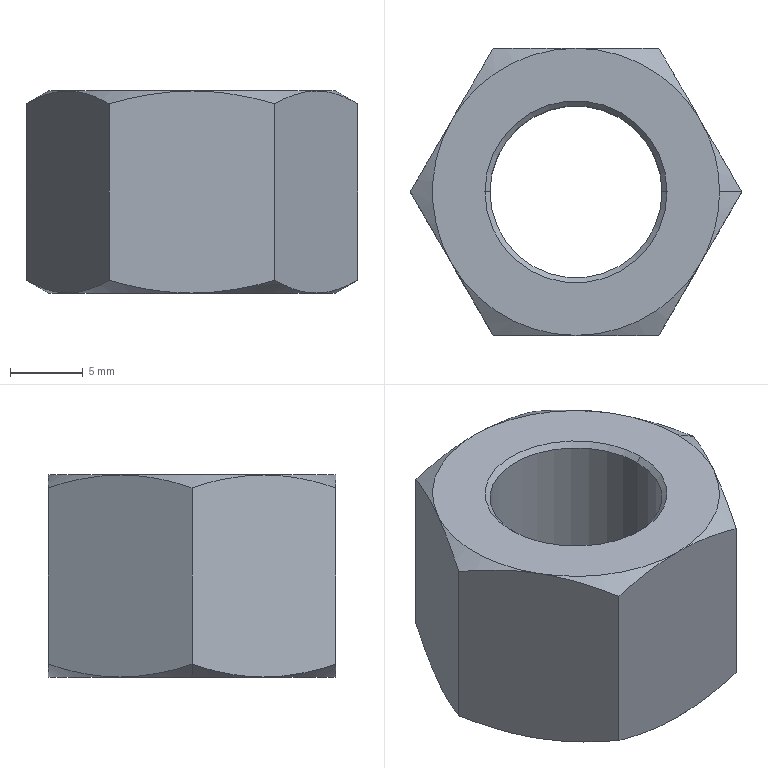Part | SolidWorks | features Cut 2, Chamfer 1, Extrusion 1 | 1 solid | 28 faces | box 22.8 x 19.745 x 13.9 mm | volume 3143 mm3 | cone 18 | plane 8 | cylinder 2 | commonest cylinder face diameters 11.835 x2
STEP:
#1=CARTESIAN_POINT('',(-5.917,0.,13.553));
#2=VERTEX_POINT('',#1);
#3=CARTESIAN_POINT('',(5.917,0.,13.553));
#4=VERTEX_POINT('',#3);
#5=CARTESIAN_POINT('',(0.,0.,13.553));
#6=DIRECTION('',(0.,0.,1.));
#7=DIRECTION('',(1.,0.,0.));
#8=AXIS2_PLACEMENT_3D('',#5,#6,#7);
#9=CIRCLE('',#8,5.917);
#10=EDGE_CURVE('',#2,#4,#9,.T.);
#11=ORIENTED_EDGE('',*,*,#10,.F.);
#12=CARTESIAN_POINT('',(-6.265,0.,13.9));
#13=VERTEX_POINT('',#12);
#14=CARTESIAN_POINT('',(-5.917,0.,13.553));
#15=DIRECTION('',(-0.7071,0.,0.7071));
#16=VECTOR('',#15,1000.);
#17=LINE('',#14,#16);
#18=EDGE_CURVE('',#2,#13,#17,.T.);
#19=ORIENTED_EDGE('',*,*,#18,.T.);
#20=CARTESIAN_POINT('',(6.265,0.,13.9));
#21=VERTEX_POINT('',#20);
#22=CARTESIAN_POINT('',(0.,0.,13.9));
#23=DIRECTION('',(0.,0.,-1.));
#24=DIRECTION('',(1.,0.,0.));
#25=AXIS2_PLACEMENT_3D('',#22,#23,#24);
#26=CIRCLE('',#25,6.265);
#27=EDGE_CURVE('',#21,#13,#26,.T.);
#28=ORIENTED_EDGE('',*,*,#27,.F.);
#29=CARTESIAN_POINT('',(5.917,0.,13.553));
#30=DIRECTION('',(0.7071,0.,0.7071));
#31=VECTOR('',#30,1000.);
#32=LINE('',#29,#31);
#33=EDGE_CURVE('',#4,#21,#32,.T.);
#34=ORIENTED_EDGE('',*,*,#33,.F.);
#35=EDGE_LOOP('',(#11,#19,#28,#34));
#36=FACE_OUTER_BOUND('',#35,.T.);
#37=CARTESIAN_POINT('',(0.,0.,13.553));
#38=DIRECTION('',(0.,0.,1.));
#39=DIRECTION('',(1.,0.,0.));
#40=AXIS2_PLACEMENT_3D('',#37,#38,#39);
#41=CONICAL_SURFACE('',#40,5.917,0.7854);
#42=ADVANCED_FACE('',(#36),#41,.F.);
#43=CARTESIAN_POINT('',(5.917,0.,0.3475));
#44=VERTEX_POINT('',#43);
#45=CARTESIAN_POINT('',(-5.917,0.,0.3475));
#46=VERTEX_POINT('',#45);
#47=CARTESIAN_POINT('',(0.,0.,0.3475));
#48=DIRECTION('',(0.,0.,-1.));
#49=DIRECTION('',(1.,0.,0.));
#50=AXIS2_PLACEMENT_3D('',#47,#48,#49);
#51=CIRCLE('',#50,5.917);
#52=EDGE_CURVE('',#44,#46,#51,.T.);
#53=ORIENTED_EDGE('',*,*,#52,.F.);
#54=CARTESIAN_POINT('',(6.265,0.,0.));
#55=VERTEX_POINT('',#54);
#56=CARTESIAN_POINT('',(6.265,0.,0.));
#57=DIRECTION('',(0.7071,0.,-0.7071));
#58=VECTOR('',#57,1000.);
#59=LINE('',#56,#58);
#60=EDGE_CURVE('',#44,#55,#59,.T.);
#61=ORIENTED_EDGE('',*,*,#60,.T.);
#62=CARTESIAN_POINT('',(-6.265,0.,0.));
#63=VERTEX_POINT('',#62);
#64=CARTESIAN_POINT('',(0.,0.,0.));
#65=DIRECTION('',(0.,0.,1.));
#66=DIRECTION('',(1.,0.,0.));
#67=AXIS2_PLACEMENT_3D('',#64,#65,#66);
#68=CIRCLE('',#67,6.265);
#69=EDGE_CURVE('',#63,#55,#68,.T.);
#70=ORIENTED_EDGE('',*,*,#69,.F.);
#71=CARTESIAN_POINT('',(-6.265,0.,0.));
#72=DIRECTION('',(-0.7071,0.,-0.7071));
#73=VECTOR('',#72,1000.);
#74=LINE('',#71,#73);
#75=EDGE_CURVE('',#46,#63,#74,.T.);
#76=ORIENTED_EDGE('',*,*,#75,.F.);
#77=EDGE_LOOP('',(#53,#61,#70,#76));
#78=FACE_OUTER_BOUND('',#77,.T.);
#79=CARTESIAN_POINT('',(0.,0.,0.));
#80=DIRECTION('',(0.,0.,-1.));
#81=DIRECTION('',(-1.,0.,0.));
#82=AXIS2_PLACEMENT_3D('',#79,#80,#81);
#83=CONICAL_SURFACE('',#82,6.265,0.7854);
#84=ADVANCED_FACE('',(#78),#83,.F.);
#85=CARTESIAN_POINT('',(9.873,0.,13.9));
#86=VERTEX_POINT('',#85);
#87=CARTESIAN_POINT('',(8.55,4.936,13.9));
#88=VERTEX_POINT('',#87);
#89=CARTESIAN_POINT('',(0.,0.,13.9));
#90=DIRECTION('',(0.,0.,1.));
#91=DIRECTION('',(1.,0.,0.));
#92=AXIS2_PLACEMENT_3D('',#89,#90,#91);
#93=CIRCLE('',#92,9.873);
#94=EDGE_CURVE('',#86,#88,#93,.T.);
#95=ORIENTED_EDGE('',*,*,#94,.F.);
#96=CARTESIAN_POINT('',(11.4,0.,13.018));
#97=VERTEX_POINT('',#96);
#98=CARTESIAN_POINT('',(9.873,0.,13.9));
#99=DIRECTION('',(0.866,0.,-0.5));
#100=VECTOR('',#99,1000.);
#101=LINE('',#98,#100);
#102=EDGE_CURVE('',#86,#97,#101,.T.);
#103=ORIENTED_EDGE('',*,*,#102,.T.);
#104=CARTESIAN_POINT('',(11.4,0.,13.018));
#105=CARTESIAN_POINT('',(10.934,0.8075,13.287));
#106=CARTESIAN_POINT('',(10.464,1.621,13.509));
#107=CARTESIAN_POINT('',(9.515,3.265,13.816));
#108=CARTESIAN_POINT('',(9.036,4.095,13.9));
#109=CARTESIAN_POINT('',(8.55,4.936,13.9));
#110=B_SPLINE_CURVE_WITH_KNOTS('',3,(#104,#105,#106,#107,#108,#109),.UNSPECIFIED.,.F.,.F.,(4,2,4),(0.000000238,0.002884,0.005768),.UNSPECIFIED.);
#111=EDGE_CURVE('',#97,#88,#110,.T.);
#112=ORIENTED_EDGE('',*,*,#111,.T.);
#113=EDGE_LOOP('',(#95,#103,#112));
#114=FACE_OUTER_BOUND('',#113,.T.);
#115=CARTESIAN_POINT('',(0.,0.,13.9));
#116=DIRECTION('',(0.,0.,-1.));
#117=DIRECTION('',(1.,0.,0.));
#118=AXIS2_PLACEMENT_3D('',#115,#116,#117);
#119=CONICAL_SURFACE('',#118,9.873,1.047);
#120=ADVANCED_FACE('',(#114),#119,.T.);
#121=CARTESIAN_POINT('',(-9.873,0.,0.));
#122=VERTEX_POINT('',#121);
#123=CARTESIAN_POINT('',(-8.55,4.936,0.));
#124=VERTEX_POINT('',#123);
#125=CARTESIAN_POINT('',(0.,0.,0.));
#126=DIRECTION('',(0.,0.,-1.));
#127=DIRECTION('',(-1.,0.,0.));
#128=AXIS2_PLACEMENT_3D('',#125,#126,#127);
#129=CIRCLE('',#128,9.873);
#130=EDGE_CURVE('',#122,#124,#129,.T.);
#131=ORIENTED_EDGE('',*,*,#130,.F.);
#132=CARTESIAN_POINT('',(-11.4,0.,0.8818));
#133=VERTEX_POINT('',#132);
#134=CARTESIAN_POINT('',(-9.873,0.,0.));
#135=DIRECTION('',(-0.866,0.,0.5));
#136=VECTOR('',#135,1000.);
#137=LINE('',#134,#136);
#138=EDGE_CURVE('',#122,#133,#137,.T.);
#139=ORIENTED_EDGE('',*,*,#138,.T.);
#140=CARTESIAN_POINT('',(-11.4,0.,0.8818));
#141=CARTESIAN_POINT('',(-10.934,0.8075,0.6126));
#142=CARTESIAN_POINT('',(-10.464,1.621,0.3909));
#143=CARTESIAN_POINT('',(-9.515,3.265,0.08404));
#144=CARTESIAN_POINT('',(-9.036,4.095,0.));
#145=CARTESIAN_POINT('',(-8.55,4.936,0.));
#146=B_SPLINE_CURVE_WITH_KNOTS('',3,(#140,#141,#142,#143,#144,#145),.UNSPECIFIED.,.F.,.F.,(4,2,4),(0.000000238,0.002884,0.005768),.UNSPECIFIED.);
#147=EDGE_CURVE('',#133,#124,#146,.T.);
#148=ORIENTED_EDGE('',*,*,#147,.T.);
#149=EDGE_LOOP('',(#131,#139,#148));
#150=FACE_OUTER_BOUND('',#149,.T.);
#151=CARTESIAN_POINT('',(0.,0.,0.));
#152=DIRECTION('',(0.,0.,1.));
#153=DIRECTION('',(-1.,0.,0.));
#154=AXIS2_PLACEMENT_3D('',#151,#152,#153);
#155=CONICAL_SURFACE('',#154,9.873,1.047);
#156=ADVANCED_FACE('',(#150),#155,.T.);
#157=ORIENTED_EDGE('',*,*,#10,.T.);
#158=CARTESIAN_POINT('',(5.917,0.,13.9));
#159=DIRECTION('',(0.,0.,-1.));
#160=VECTOR('',#159,1000.);
#161=LINE('',#158,#160);
#162=EDGE_CURVE('',#4,#44,#161,.T.);
#163=ORIENTED_EDGE('',*,*,#162,.T.);
#164=ORIENTED_EDGE('',*,*,#52,.T.);
#165=CARTESIAN_POINT('',(-5.917,0.,13.9));
#166=DIRECTION('',(0.,0.,-1.));
#167=VECTOR('',#166,1000.);
#168=LINE('',#165,#167);
#169=EDGE_CURVE('',#2,#46,#168,.T.);
#170=ORIENTED_EDGE('',*,*,#169,.F.);
#171=EDGE_LOOP('',(#157,#163,#164,#170));
#172=FACE_OUTER_BOUND('',#171,.T.);
#173=CARTESIAN_POINT('',(0.,0.,13.9));
#174=DIRECTION('',(0.,0.,-1.));
#175=DIRECTION('',(-1.,0.,0.));
#176=AXIS2_PLACEMENT_3D('',#173,#174,#175);
#177=CYLINDRICAL_SURFACE('',#176,5.917);
#178=ADVANCED_FACE('',(#172),#177,.F.);
#179=ORIENTED_EDGE('',*,*,#111,.F.);
#180=CARTESIAN_POINT('',(11.4,0.,0.8818));
#181=VERTEX_POINT('',#180);
#182=CARTESIAN_POINT('',(11.4,0.,13.9));
#183=DIRECTION('',(0.,0.,-1.));
#184=VECTOR('',#183,1000.);
#185=LINE('',#182,#184);
#186=EDGE_CURVE('',#97,#181,#185,.T.);
#187=ORIENTED_EDGE('',*,*,#186,.T.);
#188=CARTESIAN_POINT('',(8.55,4.936,0.));
#189=VERTEX_POINT('',#188);
#190=CARTESIAN_POINT('',(8.55,4.936,0.));
#191=CARTESIAN_POINT('',(8.792,4.517,0.));
#192=CARTESIAN_POINT('',(9.035,4.097,0.02084));
#193=CARTESIAN_POINT('',(9.515,3.264,0.1015));
#194=CARTESIAN_POINT('',(9.754,2.851,0.1612));
#195=CARTESIAN_POINT('',(10.466,1.618,0.3916));
#196=CARTESIAN_POINT('',(10.935,0.8055,0.6133));
#197=CARTESIAN_POINT('',(11.4,0.,0.8818));
#198=B_SPLINE_CURVE_WITH_KNOTS('',3,(#190,#191,#192,#193,#194,#195,#196,#197),.UNSPECIFIED.,.F.,.F.,(4,2,2,4),(0.005768,0.007204,0.008641,0.01151),.UNSPECIFIED.);
#199=EDGE_CURVE('',#189,#181,#198,.T.);
#200=ORIENTED_EDGE('',*,*,#199,.F.);
#201=CARTESIAN_POINT('',(5.7,9.873,0.8818));
#202=VERTEX_POINT('',#201);
#203=CARTESIAN_POINT('',(5.7,9.873,0.8818));
#204=CARTESIAN_POINT('',(6.166,9.065,0.6126));
#205=CARTESIAN_POINT('',(6.636,8.252,0.3909));
#206=CARTESIAN_POINT('',(7.585,6.608,0.08404));
#207=CARTESIAN_POINT('',(8.064,5.777,0.));
#208=CARTESIAN_POINT('',(8.55,4.936,0.));
#209=B_SPLINE_CURVE_WITH_KNOTS('',3,(#203,#204,#205,#206,#207,#208),.UNSPECIFIED.,.F.,.F.,(4,2,4),(0.000000238,0.002884,0.005768),.UNSPECIFIED.);
#210=EDGE_CURVE('',#202,#189,#209,.T.);
#211=ORIENTED_EDGE('',*,*,#210,.F.);
#212=CARTESIAN_POINT('',(5.7,9.873,13.018));
#213=VERTEX_POINT('',#212);
#214=CARTESIAN_POINT('',(5.7,9.873,13.9));
#215=DIRECTION('',(0.,0.,-1.));
#216=VECTOR('',#215,1000.);
#217=LINE('',#214,#216);
#218=EDGE_CURVE('',#213,#202,#217,.T.);
#219=ORIENTED_EDGE('',*,*,#218,.F.);
#220=CARTESIAN_POINT('',(8.55,4.936,13.9));
#221=CARTESIAN_POINT('',(8.308,5.355,13.9));
#222=CARTESIAN_POINT('',(8.065,5.776,13.879));
#223=CARTESIAN_POINT('',(7.585,6.609,13.799));
#224=CARTESIAN_POINT('',(7.346,7.022,13.739));
#225=CARTESIAN_POINT('',(6.634,8.255,13.508));
#226=CARTESIAN_POINT('',(6.165,9.067,13.287));
#227=CARTESIAN_POINT('',(5.7,9.873,13.018));
#228=B_SPLINE_CURVE_WITH_KNOTS('',3,(#220,#221,#222,#223,#224,#225,#226,#227),.UNSPECIFIED.,.F.,.F.,(4,2,2,4),(0.005768,0.007204,0.008641,0.01151),.UNSPECIFIED.);
#229=EDGE_CURVE('',#88,#213,#228,.T.);
#230=ORIENTED_EDGE('',*,*,#229,.F.);
#231=EDGE_LOOP('',(#179,#187,#200,#211,#219,#230));
#232=FACE_OUTER_BOUND('',#231,.T.);
#233=CARTESIAN_POINT('',(11.4,0.,13.9));
#234=DIRECTION('',(-0.866,-0.5,0.));
#235=DIRECTION('',(0.5,-0.866,0.));
#236=AXIS2_PLACEMENT_3D('',#233,#234,#235);
#237=PLANE('',#236);
#238=ADVANCED_FACE('',(#232),#237,.F.);
#239=CARTESIAN_POINT('',(0.,9.873,13.9));
#240=VERTEX_POINT('',#239);
#241=CARTESIAN_POINT('',(5.7,9.873,13.018));
#242=CARTESIAN_POINT('',(4.778,9.873,13.284));
#243=CARTESIAN_POINT('',(3.845,9.873,13.506));
#244=CARTESIAN_POINT('',(2.418,9.873,13.737));
#245=CARTESIAN_POINT('',(1.938,9.873,13.798));
#246=CARTESIAN_POINT('',(0.9674,9.873,13.879));
#247=CARTESIAN_POINT('',(0.4824,9.873,13.9));
#248=CARTESIAN_POINT('',(0.,9.873,13.9));
#249=B_SPLINE_CURVE_WITH_KNOTS('',3,(#241,#242,#243,#244,#245,#246,#247,#248),.UNSPECIFIED.,.F.,.F.,(4,2,2,4),(0.03412,0.03701,0.03845,0.03989),.UNSPECIFIED.);
#250=EDGE_CURVE('',#213,#240,#249,.T.);
#251=ORIENTED_EDGE('',*,*,#250,.F.);
#252=ORIENTED_EDGE('',*,*,#218,.T.);
#253=CARTESIAN_POINT('',(0.,9.873,0.));
#254=VERTEX_POINT('',#253);
#255=CARTESIAN_POINT('',(0.,9.873,0.));
#256=CARTESIAN_POINT('',(0.4824,9.873,0.));
#257=CARTESIAN_POINT('',(0.9674,9.873,0.02059));
#258=CARTESIAN_POINT('',(1.938,9.873,0.1021));
#259=CARTESIAN_POINT('',(2.418,9.873,0.1625));
#260=CARTESIAN_POINT('',(3.845,9.873,0.3942));
#261=CARTESIAN_POINT('',(4.778,9.873,0.6157));
#262=CARTESIAN_POINT('',(5.7,9.873,0.8818));
#263=B_SPLINE_CURVE_WITH_KNOTS('',3,(#255,#256,#257,#258,#259,#260,#261,#262),.UNSPECIFIED.,.F.,.F.,(4,2,2,4),(0.01627,0.01771,0.01915,0.02204),.UNSPECIFIED.);
#264=EDGE_CURVE('',#254,#202,#263,.T.);
#265=ORIENTED_EDGE('',*,*,#264,.F.);
#266=CARTESIAN_POINT('',(-5.7,9.873,0.8818));
#267=VERTEX_POINT('',#266);
#268=CARTESIAN_POINT('',(-5.7,9.873,0.8818));
#269=CARTESIAN_POINT('',(-4.772,9.873,0.6139));
#270=CARTESIAN_POINT('',(-3.823,9.873,0.3896));
#271=CARTESIAN_POINT('',(-1.921,9.873,0.08294));
#272=CARTESIAN_POINT('',(-0.9642,9.873,0.));
#273=CARTESIAN_POINT('',(0.,9.873,0.));
#274=B_SPLINE_CURVE_WITH_KNOTS('',3,(#268,#269,#270,#271,#272,#273),.UNSPECIFIED.,.F.,.F.,(4,2,4),(0.0105,0.01338,0.01627),.UNSPECIFIED.);
#275=EDGE_CURVE('',#267,#254,#274,.T.);
#276=ORIENTED_EDGE('',*,*,#275,.F.);
#277=CARTESIAN_POINT('',(-5.7,9.873,13.018));
#278=VERTEX_POINT('',#277);
#279=CARTESIAN_POINT('',(-5.7,9.873,13.9));
#280=DIRECTION('',(0.,0.,-1.));
#281=VECTOR('',#280,1000.);
#282=LINE('',#279,#281);
#283=EDGE_CURVE('',#278,#267,#282,.T.);
#284=ORIENTED_EDGE('',*,*,#283,.F.);
#285=CARTESIAN_POINT('',(0.,9.873,13.9));
#286=CARTESIAN_POINT('',(-0.9642,9.873,13.9));
#287=CARTESIAN_POINT('',(-1.921,9.873,13.817));
#288=CARTESIAN_POINT('',(-3.823,9.873,13.51));
#289=CARTESIAN_POINT('',(-4.772,9.873,13.286));
#290=CARTESIAN_POINT('',(-5.7,9.873,13.018));
#291=B_SPLINE_CURVE_WITH_KNOTS('',3,(#285,#286,#287,#288,#289,#290),.UNSPECIFIED.,.F.,.F.,(4,2,4),(0.03989,0.04277,0.04566),.UNSPECIFIED.);
#292=EDGE_CURVE('',#240,#278,#291,.T.);
#293=ORIENTED_EDGE('',*,*,#292,.F.);
#294=EDGE_LOOP('',(#251,#252,#265,#276,#284,#293));
#295=FACE_OUTER_BOUND('',#294,.T.);
#296=CARTESIAN_POINT('',(5.7,9.873,13.9));
#297=DIRECTION('',(0.,-1.,0.));
#298=DIRECTION('',(1.,0.,0.));
#299=AXIS2_PLACEMENT_3D('',#296,#297,#298);
#300=PLANE('',#299);
#301=ADVANCED_FACE('',(#295),#300,.F.);
#302=CARTESIAN_POINT('',(-8.55,4.936,13.9));
#303=VERTEX_POINT('',#302);
#304=CARTESIAN_POINT('',(-5.7,9.873,13.018));
#305=CARTESIAN_POINT('',(-6.166,9.065,13.287));
#306=CARTESIAN_POINT('',(-6.636,8.252,13.509));
#307=CARTESIAN_POINT('',(-7.585,6.608,13.816));
#308=CARTESIAN_POINT('',(-8.064,5.777,13.9));
#309=CARTESIAN_POINT('',(-8.55,4.936,13.9));
#310=B_SPLINE_CURVE_WITH_KNOTS('',3,(#304,#305,#306,#307,#308,#309),.UNSPECIFIED.,.F.,.F.,(4,2,4),(0.000000238,0.002884,0.005768),.UNSPECIFIED.);
#311=EDGE_CURVE('',#278,#303,#310,.T.);
#312=ORIENTED_EDGE('',*,*,#311,.F.);
#313=ORIENTED_EDGE('',*,*,#283,.T.);
#314=CARTESIAN_POINT('',(-8.55,4.936,0.));
#315=CARTESIAN_POINT('',(-8.308,5.355,0.));
#316=CARTESIAN_POINT('',(-8.065,5.776,0.02084));
#317=CARTESIAN_POINT('',(-7.585,6.609,0.1015));
#318=CARTESIAN_POINT('',(-7.346,7.022,0.1612));
#319=CARTESIAN_POINT('',(-6.634,8.255,0.3916));
#320=CARTESIAN_POINT('',(-6.165,9.067,0.6133));
#321=CARTESIAN_POINT('',(-5.7,9.873,0.8818));
#322=B_SPLINE_CURVE_WITH_KNOTS('',3,(#314,#315,#316,#317,#318,#319,#320,#321),.UNSPECIFIED.,.F.,.F.,(4,2,2,4),(0.005768,0.007204,0.008641,0.01151),.UNSPECIFIED.);
#323=EDGE_CURVE('',#124,#267,#322,.T.);
#324=ORIENTED_EDGE('',*,*,#323,.F.);
#325=ORIENTED_EDGE('',*,*,#147,.F.);
#326=CARTESIAN_POINT('',(-11.4,0.,13.018));
#327=VERTEX_POINT('',#326);
#328=CARTESIAN_POINT('',(-11.4,0.,13.9));
#329=DIRECTION('',(0.,0.,-1.));
#330=VECTOR('',#329,1000.);
#331=LINE('',#328,#330);
#332=EDGE_CURVE('',#327,#133,#331,.T.);
#333=ORIENTED_EDGE('',*,*,#332,.F.);
#334=CARTESIAN_POINT('',(-8.55,4.936,13.9));
#335=CARTESIAN_POINT('',(-8.792,4.517,13.9));
#336=CARTESIAN_POINT('',(-9.035,4.097,13.879));
#337=CARTESIAN_POINT('',(-9.515,3.264,13.799));
#338=CARTESIAN_POINT('',(-9.754,2.851,13.739));
#339=CARTESIAN_POINT('',(-10.466,1.618,13.508));
#340=CARTESIAN_POINT('',(-10.935,0.8055,13.287));
#341=CARTESIAN_POINT('',(-11.4,0.,13.018));
#342=B_SPLINE_CURVE_WITH_KNOTS('',3,(#334,#335,#336,#337,#338,#339,#340,#341),.UNSPECIFIED.,.F.,.F.,(4,2,2,4),(0.005768,0.007204,0.008641,0.01151),.UNSPECIFIED.);
#343=EDGE_CURVE('',#303,#327,#342,.T.);
#344=ORIENTED_EDGE('',*,*,#343,.F.);
#345=EDGE_LOOP('',(#312,#313,#324,#325,#333,#344));
#346=FACE_OUTER_BOUND('',#345,.T.);
#347=CARTESIAN_POINT('',(-5.7,9.873,13.9));
#348=DIRECTION('',(0.866,-0.5,0.));
#349=DIRECTION('',(0.5,0.866,0.));
#350=AXIS2_PLACEMENT_3D('',#347,#348,#349);
#351=PLANE('',#350);
#352=ADVANCED_FACE('',(#346),#351,.F.);
#353=CARTESIAN_POINT('',(-8.55,-4.936,13.9));
#354=VERTEX_POINT('',#353);
#355=CARTESIAN_POINT('',(-11.4,0.,13.018));
#356=CARTESIAN_POINT('',(-10.934,-0.8075,13.287));
#357=CARTESIAN_POINT('',(-10.464,-1.621,13.509));
#358=CARTESIAN_POINT('',(-9.515,-3.265,13.816));
#359=CARTESIAN_POINT('',(-9.036,-4.095,13.9));
#360=CARTESIAN_POINT('',(-8.55,-4.936,13.9));
#361=B_SPLINE_CURVE_WITH_KNOTS('',3,(#355,#356,#357,#358,#359,#360),.UNSPECIFIED.,.F.,.F.,(4,2,4),(0.000000238,0.002884,0.005768),.UNSPECIFIED.);
#362=EDGE_CURVE('',#327,#354,#361,.T.);
#363=ORIENTED_EDGE('',*,*,#362,.F.);
#364=ORIENTED_EDGE('',*,*,#332,.T.);
#365=CARTESIAN_POINT('',(-8.55,-4.936,0.));
#366=VERTEX_POINT('',#365);
#367=CARTESIAN_POINT('',(-8.55,-4.936,0.));
#368=CARTESIAN_POINT('',(-8.792,-4.517,0.));
#369=CARTESIAN_POINT('',(-9.035,-4.097,0.02084));
#370=CARTESIAN_POINT('',(-9.515,-3.264,0.1015));
#371=CARTESIAN_POINT('',(-9.754,-2.851,0.1612));
#372=CARTESIAN_POINT('',(-10.466,-1.618,0.3916));
#373=CARTESIAN_POINT('',(-10.935,-0.8055,0.6133));
#374=CARTESIAN_POINT('',(-11.4,0.,0.8818));
#375=B_SPLINE_CURVE_WITH_KNOTS('',3,(#367,#368,#369,#370,#371,#372,#373,#374),.UNSPECIFIED.,.F.,.F.,(4,2,2,4),(0.005768,0.007204,0.008641,0.01151),.UNSPECIFIED.);
#376=EDGE_CURVE('',#366,#133,#375,.T.);
#377=ORIENTED_EDGE('',*,*,#376,.F.);
#378=CARTESIAN_POINT('',(-5.7,-9.873,0.8818));
#379=VERTEX_POINT('',#378);
#380=CARTESIAN_POINT('',(-5.7,-9.873,0.8818));
#381=CARTESIAN_POINT('',(-6.166,-9.065,0.6126));
#382=CARTESIAN_POINT('',(-6.636,-8.252,0.3909));
#383=CARTESIAN_POINT('',(-7.585,-6.608,0.08404));
#384=CARTESIAN_POINT('',(-8.064,-5.777,0.));
#385=CARTESIAN_POINT('',(-8.55,-4.936,0.));
#386=B_SPLINE_CURVE_WITH_KNOTS('',3,(#380,#381,#382,#383,#384,#385),.UNSPECIFIED.,.F.,.F.,(4,2,4),(0.000000238,0.002884,0.005768),.UNSPECIFIED.);
#387=EDGE_CURVE('',#379,#366,#386,.T.);
#388=ORIENTED_EDGE('',*,*,#387,.F.);
#389=CARTESIAN_POINT('',(-5.7,-9.873,13.018));
#390=VERTEX_POINT('',#389);
#391=CARTESIAN_POINT('',(-5.7,-9.873,13.9));
#392=DIRECTION('',(0.,0.,-1.));
#393=VECTOR('',#392,1000.);
#394=LINE('',#391,#393);
#395=EDGE_CURVE('',#390,#379,#394,.T.);
#396=ORIENTED_EDGE('',*,*,#395,.F.);
#397=CARTESIAN_POINT('',(-8.55,-4.936,13.9));
#398=CARTESIAN_POINT('',(-8.308,-5.355,13.9));
#399=CARTESIAN_POINT('',(-8.065,-5.776,13.879));
#400=CARTESIAN_POINT('',(-7.585,-6.609,13.799));
#401=CARTESIAN_POINT('',(-7.346,-7.022,13.739));
#402=CARTESIAN_POINT('',(-6.634,-8.255,13.508));
#403=CARTESIAN_POINT('',(-6.165,-9.067,13.287));
#404=CARTESIAN_POINT('',(-5.7,-9.873,13.018));
#405=B_SPLINE_CURVE_WITH_KNOTS('',3,(#397,#398,#399,#400,#401,#402,#403,#404),.UNSPECIFIED.,.F.,.F.,(4,2,2,4),(0.005768,0.007204,0.008641,0.01151),.UNSPECIFIED.);
#406=EDGE_CURVE('',#354,#390,#405,.T.);
#407=ORIENTED_EDGE('',*,*,#406,.F.);
#408=EDGE_LOOP('',(#363,#364,#377,#388,#396,#407));
#409=FACE_OUTER_BOUND('',#408,.T.);
#410=CARTESIAN_POINT('',(-11.4,0.,13.9));
#411=DIRECTION('',(0.866,0.5,0.));
#412=DIRECTION('',(-0.5,0.866,0.));
#413=AXIS2_PLACEMENT_3D('',#410,#411,#412);
#414=PLANE('',#413);
#415=ADVANCED_FACE('',(#409),#414,.F.);
#416=CARTESIAN_POINT('',(0.,-9.873,13.9));
#417=VERTEX_POINT('',#416);
#418=CARTESIAN_POINT('',(-5.7,-9.873,13.018));
#419=CARTESIAN_POINT('',(-4.772,-9.873,13.286));
#420=CARTESIAN_POINT('',(-3.823,-9.873,13.51));
#421=CARTESIAN_POINT('',(-1.921,-9.873,13.817));
#422=CARTESIAN_POINT('',(-0.9642,-9.873,13.9));
#423=CARTESIAN_POINT('',(0.,-9.873,13.9));
#424=B_SPLINE_CURVE_WITH_KNOTS('',3,(#418,#419,#420,#421,#422,#423),.UNSPECIFIED.,.F.,.F.,(4,2,4),(0.0105,0.01338,0.01627),.UNSPECIFIED.);
#425=EDGE_CURVE('',#390,#417,#424,.T.);
#426=ORIENTED_EDGE('',*,*,#425,.F.);
#427=ORIENTED_EDGE('',*,*,#395,.T.);
#428=CARTESIAN_POINT('',(0.,-9.873,0.));
#429=VERTEX_POINT('',#428);
#430=CARTESIAN_POINT('',(0.,-9.873,0.));
#431=CARTESIAN_POINT('',(-0.9642,-9.873,0.));
#432=CARTESIAN_POINT('',(-1.921,-9.873,0.08294));
#433=CARTESIAN_POINT('',(-3.823,-9.873,0.3896));
#434=CARTESIAN_POINT('',(-4.772,-9.873,0.6139));
#435=CARTESIAN_POINT('',(-5.7,-9.873,0.8818));
#436=B_SPLINE_CURVE_WITH_KNOTS('',3,(#430,#431,#432,#433,#434,#435),.UNSPECIFIED.,.F.,.F.,(4,2,4),(0.03989,0.04277,0.04566),.UNSPECIFIED.);
#437=EDGE_CURVE('',#429,#379,#436,.T.);
#438=ORIENTED_EDGE('',*,*,#437,.F.);
#439=CARTESIAN_POINT('',(5.7,-9.873,0.8818));
#440=VERTEX_POINT('',#439);
#441=CARTESIAN_POINT('',(5.7,-9.873,0.8818));
#442=CARTESIAN_POINT('',(4.778,-9.873,0.6157));
#443=CARTESIAN_POINT('',(3.845,-9.873,0.3942));
#444=CARTESIAN_POINT('',(2.418,-9.873,0.1625));
#445=CARTESIAN_POINT('',(1.938,-9.873,0.1021));
#446=CARTESIAN_POINT('',(0.9674,-9.873,0.02059));
#447=CARTESIAN_POINT('',(0.4824,-9.873,0.));
#448=CARTESIAN_POINT('',(0.,-9.873,0.));
#449=B_SPLINE_CURVE_WITH_KNOTS('',3,(#441,#442,#443,#444,#445,#446,#447,#448),.UNSPECIFIED.,.F.,.F.,(4,2,2,4),(0.03412,0.03701,0.03845,0.03989),.UNSPECIFIED.);
#450=EDGE_CURVE('',#440,#429,#449,.T.);
#451=ORIENTED_EDGE('',*,*,#450,.F.);
#452=CARTESIAN_POINT('',(5.7,-9.873,13.018));
#453=VERTEX_POINT('',#452);
#454=CARTESIAN_POINT('',(5.7,-9.873,13.9));
#455=DIRECTION('',(0.,0.,-1.));
#456=VECTOR('',#455,1000.);
#457=LINE('',#454,#456);
#458=EDGE_CURVE('',#453,#440,#457,.T.);
#459=ORIENTED_EDGE('',*,*,#458,.F.);
#460=CARTESIAN_POINT('',(0.,-9.873,13.9));
#461=CARTESIAN_POINT('',(0.4824,-9.873,13.9));
#462=CARTESIAN_POINT('',(0.9674,-9.873,13.879));
#463=CARTESIAN_POINT('',(1.938,-9.873,13.798));
#464=CARTESIAN_POINT('',(2.418,-9.873,13.737));
#465=CARTESIAN_POINT('',(3.845,-9.873,13.506));
#466=CARTESIAN_POINT('',(4.778,-9.873,13.284));
#467=CARTESIAN_POINT('',(5.7,-9.873,13.018));
#468=B_SPLINE_CURVE_WITH_KNOTS('',3,(#460,#461,#462,#463,#464,#465,#466,#467),.UNSPECIFIED.,.F.,.F.,(4,2,2,4),(0.01627,0.01771,0.01915,0.02204),.UNSPECIFIED.);
#469=EDGE_CURVE('',#417,#453,#468,.T.);
#470=ORIENTED_EDGE('',*,*,#469,.F.);
#471=EDGE_LOOP('',(#426,#427,#438,#451,#459,#470));
#472=FACE_OUTER_BOUND('',#471,.T.);
#473=CARTESIAN_POINT('',(-5.7,-9.873,13.9));
#474=DIRECTION('',(0.,1.,0.));
#475=DIRECTION('',(0.,0.,1.));
#476=AXIS2_PLACEMENT_3D('',#473,#474,#475);
#477=PLANE('',#476);
#478=ADVANCED_FACE('',(#472),#477,.F.);
#479=CARTESIAN_POINT('',(8.55,-4.936,13.9));
#480=VERTEX_POINT('',#479);
#481=CARTESIAN_POINT('',(5.7,-9.873,13.018));
#482=CARTESIAN_POINT('',(6.166,-9.065,13.287));
#483=CARTESIAN_POINT('',(6.636,-8.252,13.509));
#484=CARTESIAN_POINT('',(7.585,-6.608,13.816));
#485=CARTESIAN_POINT('',(8.064,-5.777,13.9));
#486=CARTESIAN_POINT('',(8.55,-4.936,13.9));
#487=B_SPLINE_CURVE_WITH_KNOTS('',3,(#481,#482,#483,#484,#485,#486),.UNSPECIFIED.,.F.,.F.,(4,2,4),(0.000000238,0.002884,0.005768),.UNSPECIFIED.);
#488=EDGE_CURVE('',#453,#480,#487,.T.);
#489=ORIENTED_EDGE('',*,*,#488,.F.);
#490=ORIENTED_EDGE('',*,*,#458,.T.);
#491=CARTESIAN_POINT('',(8.55,-4.936,0.));
#492=VERTEX_POINT('',#491);
#493=CARTESIAN_POINT('',(8.55,-4.936,0.));
#494=CARTESIAN_POINT('',(8.308,-5.355,0.));
#495=CARTESIAN_POINT('',(8.065,-5.776,0.02084));
#496=CARTESIAN_POINT('',(7.585,-6.609,0.1015));
#497=CARTESIAN_POINT('',(7.346,-7.022,0.1612));
#498=CARTESIAN_POINT('',(6.634,-8.255,0.3916));
#499=CARTESIAN_POINT('',(6.165,-9.067,0.6133));
#500=CARTESIAN_POINT('',(5.7,-9.873,0.8818));
#501=B_SPLINE_CURVE_WITH_KNOTS('',3,(#493,#494,#495,#496,#497,#498,#499,#500),.UNSPECIFIED.,.F.,.F.,(4,2,2,4),(0.005768,0.007204,0.008641,0.01151),.UNSPECIFIED.);
#502=EDGE_CURVE('',#492,#440,#501,.T.);
#503=ORIENTED_EDGE('',*,*,#502,.F.);
#504=CARTESIAN_POINT('',(11.4,0.,0.8818));
#505=CARTESIAN_POINT('',(10.934,-0.8075,0.6126));
#506=CARTESIAN_POINT('',(10.464,-1.621,0.3909));
#507=CARTESIAN_POINT('',(9.515,-3.265,0.08404));
#508=CARTESIAN_POINT('',(9.036,-4.095,0.));
#509=CARTESIAN_POINT('',(8.55,-4.936,0.));
#510=B_SPLINE_CURVE_WITH_KNOTS('',3,(#504,#505,#506,#507,#508,#509),.UNSPECIFIED.,.F.,.F.,(4,2,4),(0.000000238,0.002884,0.005768),.UNSPECIFIED.);
#511=EDGE_CURVE('',#181,#492,#510,.T.);
#512=ORIENTED_EDGE('',*,*,#511,.F.);
#513=ORIENTED_EDGE('',*,*,#186,.F.);
#514=CARTESIAN_POINT('',(8.55,-4.936,13.9));
#515=CARTESIAN_POINT('',(8.792,-4.517,13.9));
#516=CARTESIAN_POINT('',(9.035,-4.097,13.879));
#517=CARTESIAN_POINT('',(9.515,-3.264,13.799));
#518=CARTESIAN_POINT('',(9.754,-2.851,13.739));
#519=CARTESIAN_POINT('',(10.466,-1.618,13.508));
#520=CARTESIAN_POINT('',(10.935,-0.8055,13.287));
#521=CARTESIAN_POINT('',(11.4,0.,13.018));
#522=B_SPLINE_CURVE_WITH_KNOTS('',3,(#514,#515,#516,#517,#518,#519,#520,#521),.UNSPECIFIED.,.F.,.F.,(4,2,2,4),(0.005768,0.007204,0.008641,0.01151),.UNSPECIFIED.);
#523=EDGE_CURVE('',#480,#97,#522,.T.);
#524=ORIENTED_EDGE('',*,*,#523,.F.);
#525=EDGE_LOOP('',(#489,#490,#503,#512,#513,#524));
#526=FACE_OUTER_BOUND('',#525,.T.);
#527=CARTESIAN_POINT('',(5.7,-9.873,13.9));
#528=DIRECTION('',(-0.866,0.5,0.));
#529=DIRECTION('',(-0.5,-0.866,0.));
#530=AXIS2_PLACEMENT_3D('',#527,#528,#529);
#531=PLANE('',#530);
#532=ADVANCED_FACE('',(#526),#531,.F.);
#533=ORIENTED_EDGE('',*,*,#27,.T.);
#534=CARTESIAN_POINT('',(0.,0.,13.9));
#535=DIRECTION('',(0.,0.,-1.));
#536=DIRECTION('',(1.,0.,0.));
#537=AXIS2_PLACEMENT_3D('',#534,#535,#536);
#538=CIRCLE('',#537,6.265);
#539=EDGE_CURVE('',#13,#21,#538,.T.);
#540=ORIENTED_EDGE('',*,*,#539,.T.);
#541=EDGE_LOOP('',(#533,#540));
#542=FACE_BOUND('',#541,.T.);
#543=CARTESIAN_POINT('',(0.,0.,13.9));
#544=DIRECTION('',(0.,0.,1.));
#545=DIRECTION('',(1.,0.,0.));
#546=AXIS2_PLACEMENT_3D('',#543,#544,#545);
#547=CIRCLE('',#546,9.873);
#548=EDGE_CURVE('',#480,#86,#547,.T.);
#549=ORIENTED_EDGE('',*,*,#548,.T.);
#550=ORIENTED_EDGE('',*,*,#94,.T.);
#551=CARTESIAN_POINT('',(0.,0.,13.9));
#552=DIRECTION('',(0.,0.,1.));
#553=DIRECTION('',(1.,0.,0.));
#554=AXIS2_PLACEMENT_3D('',#551,#552,#553);
#555=CIRCLE('',#554,9.873);
#556=EDGE_CURVE('',#88,#240,#555,.T.);
#557=ORIENTED_EDGE('',*,*,#556,.T.);
#558=CARTESIAN_POINT('',(0.,0.,13.9));
#559=DIRECTION('',(0.,0.,1.));
#560=DIRECTION('',(1.,0.,0.));
#561=AXIS2_PLACEMENT_3D('',#558,#559,#560);
#562=CIRCLE('',#561,9.873);
#563=EDGE_CURVE('',#240,#303,#562,.T.);
#564=ORIENTED_EDGE('',*,*,#563,.T.);
#565=CARTESIAN_POINT('',(0.,0.,13.9));
#566=DIRECTION('',(0.,0.,1.));
#567=DIRECTION('',(1.,0.,0.));
#568=AXIS2_PLACEMENT_3D('',#565,#566,#567);
#569=CIRCLE('',#568,9.873);
#570=EDGE_CURVE('',#303,#354,#569,.T.);
#571=ORIENTED_EDGE('',*,*,#570,.T.);
#572=CARTESIAN_POINT('',(0.,0.,13.9));
#573=DIRECTION('',(0.,0.,1.));
#574=DIRECTION('',(1.,0.,0.));
#575=AXIS2_PLACEMENT_3D('',#572,#573,#574);
#576=CIRCLE('',#575,9.873);
#577=EDGE_CURVE('',#354,#417,#576,.T.);
#578=ORIENTED_EDGE('',*,*,#577,.T.);
#579=CARTESIAN_POINT('',(0.,0.,13.9));
#580=DIRECTION('',(0.,0.,1.));
#581=DIRECTION('',(1.,0.,0.));
#582=AXIS2_PLACEMENT_3D('',#579,#580,#581);
#583=CIRCLE('',#582,9.873);
#584=EDGE_CURVE('',#417,#480,#583,.T.);
#585=ORIENTED_EDGE('',*,*,#584,.T.);
#586=EDGE_LOOP('',(#549,#550,#557,#564,#571,#578,#585));
#587=FACE_OUTER_BOUND('',#586,.T.);
#588=CARTESIAN_POINT('',(0.,19.745,13.9));
#589=DIRECTION('',(0.,0.,1.));
#590=DIRECTION('',(1.,0.,0.));
#591=AXIS2_PLACEMENT_3D('',#588,#589,#590);
#592=PLANE('',#591);
#593=ADVANCED_FACE('',(#542,#587),#592,.T.);
#594=ORIENTED_EDGE('',*,*,#69,.T.);
#595=CARTESIAN_POINT('',(0.,0.,0.));
#596=DIRECTION('',(0.,0.,1.));
#597=DIRECTION('',(1.,0.,0.));
#598=AXIS2_PLACEMENT_3D('',#595,#596,#597);
#599=CIRCLE('',#598,6.265);
#600=EDGE_CURVE('',#55,#63,#599,.T.);
#601=ORIENTED_EDGE('',*,*,#600,.T.);
#602=EDGE_LOOP('',(#594,#601));
#603=FACE_BOUND('',#602,.T.);
#604=CARTESIAN_POINT('',(0.,0.,0.));
#605=DIRECTION('',(0.,0.,-1.));
#606=DIRECTION('',(-1.,0.,0.));
#607=AXIS2_PLACEMENT_3D('',#604,#605,#606);
#608=CIRCLE('',#607,9.873);
#609=EDGE_CURVE('',#254,#189,#608,.T.);
#610=ORIENTED_EDGE('',*,*,#609,.T.);
#611=CARTESIAN_POINT('',(0.,0.,0.));
#612=DIRECTION('',(0.,0.,-1.));
#613=DIRECTION('',(-1.,0.,0.));
#614=AXIS2_PLACEMENT_3D('',#611,#612,#613);
#615=CIRCLE('',#614,9.873);
#616=EDGE_CURVE('',#189,#492,#615,.T.);
#617=ORIENTED_EDGE('',*,*,#616,.T.);
#618=CARTESIAN_POINT('',(0.,0.,0.));
#619=DIRECTION('',(0.,0.,-1.));
#620=DIRECTION('',(-1.,0.,0.));
#621=AXIS2_PLACEMENT_3D('',#618,#619,#620);
#622=CIRCLE('',#621,9.873);
#623=EDGE_CURVE('',#492,#429,#622,.T.);
#624=ORIENTED_EDGE('',*,*,#623,.T.);
#625=CARTESIAN_POINT('',(0.,0.,0.));
#626=DIRECTION('',(0.,0.,-1.));
#627=DIRECTION('',(-1.,0.,0.));
#628=AXIS2_PLACEMENT_3D('',#625,#626,#627);
#629=CIRCLE('',#628,9.873);
#630=EDGE_CURVE('',#429,#366,#629,.T.);
#631=ORIENTED_EDGE('',*,*,#630,.T.);
#632=CARTESIAN_POINT('',(0.,0.,0.));
#633=DIRECTION('',(0.,0.,-1.));
#634=DIRECTION('',(-1.,0.,0.));
#635=AXIS2_PLACEMENT_3D('',#632,#633,#634);
#636=CIRCLE('',#635,9.873);
#637=EDGE_CURVE('',#366,#122,#636,.T.);
#638=ORIENTED_EDGE('',*,*,#637,.T.);
#639=ORIENTED_EDGE('',*,*,#130,.T.);
#640=CARTESIAN_POINT('',(0.,0.,0.));
#641=DIRECTION('',(0.,0.,-1.));
#642=DIRECTION('',(-1.,0.,0.));
#643=AXIS2_PLACEMENT_3D('',#640,#641,#642);
#644=CIRCLE('',#643,9.873);
#645=EDGE_CURVE('',#124,#254,#644,.T.);
#646=ORIENTED_EDGE('',*,*,#645,.T.);
#647=EDGE_LOOP('',(#610,#617,#624,#631,#638,#639,#646));
#648=FACE_OUTER_BOUND('',#647,.T.);
#649=CARTESIAN_POINT('',(0.,19.745,0.));
#650=DIRECTION('',(0.,0.,1.));
#651=DIRECTION('',(1.,0.,0.));
#652=AXIS2_PLACEMENT_3D('',#649,#650,#651);
#653=PLANE('',#652);
#654=ADVANCED_FACE('',(#603,#648),#653,.F.);
#655=ORIENTED_EDGE('',*,*,#162,.F.);
#656=CARTESIAN_POINT('',(0.,0.,13.553));
#657=DIRECTION('',(0.,0.,1.));
#658=DIRECTION('',(1.,0.,0.));
#659=AXIS2_PLACEMENT_3D('',#656,#657,#658);
#660=CIRCLE('',#659,5.917);
#661=EDGE_CURVE('',#4,#2,#660,.T.);
#662=ORIENTED_EDGE('',*,*,#661,.T.);
#663=ORIENTED_EDGE('',*,*,#169,.T.);
#664=CARTESIAN_POINT('',(0.,0.,0.3475));
#665=DIRECTION('',(0.,0.,-1.));
#666=DIRECTION('',(1.,0.,0.));
#667=AXIS2_PLACEMENT_3D('',#664,#665,#666);
#668=CIRCLE('',#667,5.917);
#669=EDGE_CURVE('',#46,#44,#668,.T.);
#670=ORIENTED_EDGE('',*,*,#669,.T.);
#671=EDGE_LOOP('',(#655,#662,#663,#670));
#672=FACE_OUTER_BOUND('',#671,.T.);
#673=CARTESIAN_POINT('',(0.,0.,13.9));
#674=DIRECTION('',(0.,0.,-1.));
#675=DIRECTION('',(-1.,0.,0.));
#676=AXIS2_PLACEMENT_3D('',#673,#674,#675);
#677=CYLINDRICAL_SURFACE('',#676,5.917);
#678=ADVANCED_FACE('',(#672),#677,.F.);
#679=ORIENTED_EDGE('',*,*,#450,.T.);
#680=ORIENTED_EDGE('',*,*,#623,.F.);
#681=ORIENTED_EDGE('',*,*,#502,.T.);
#682=EDGE_LOOP('',(#679,#680,#681));
#683=FACE_OUTER_BOUND('',#682,.T.);
#684=CARTESIAN_POINT('',(0.,0.,0.));
#685=DIRECTION('',(0.,0.,1.));
#686=DIRECTION('',(-1.,0.,0.));
#687=AXIS2_PLACEMENT_3D('',#684,#685,#686);
#688=CONICAL_SURFACE('',#687,9.873,1.047);
#689=ADVANCED_FACE('',(#683),#688,.T.);
#690=ORIENTED_EDGE('',*,*,#199,.T.);
#691=ORIENTED_EDGE('',*,*,#511,.T.);
#692=ORIENTED_EDGE('',*,*,#616,.F.);
#693=EDGE_LOOP('',(#690,#691,#692));
#694=FACE_OUTER_BOUND('',#693,.T.);
#695=CARTESIAN_POINT('',(0.,0.,0.));
#696=DIRECTION('',(0.,0.,1.));
#697=DIRECTION('',(-1.,0.,0.));
#698=AXIS2_PLACEMENT_3D('',#695,#696,#697);
#699=CONICAL_SURFACE('',#698,9.873,1.047);
#700=ADVANCED_FACE('',(#694),#699,.T.);
#701=ORIENTED_EDGE('',*,*,#387,.T.);
#702=ORIENTED_EDGE('',*,*,#630,.F.);
#703=ORIENTED_EDGE('',*,*,#437,.T.);
#704=EDGE_LOOP('',(#701,#702,#703));
#705=FACE_OUTER_BOUND('',#704,.T.);
#706=CARTESIAN_POINT('',(0.,0.,0.));
#707=DIRECTION('',(0.,0.,1.));
#708=DIRECTION('',(-1.,0.,0.));
#709=AXIS2_PLACEMENT_3D('',#706,#707,#708);
#710=CONICAL_SURFACE('',#709,9.873,1.047);
#711=ADVANCED_FACE('',(#705),#710,.T.);
#712=ORIENTED_EDGE('',*,*,#138,.F.);
#713=ORIENTED_EDGE('',*,*,#637,.F.);
#714=ORIENTED_EDGE('',*,*,#376,.T.);
#715=EDGE_LOOP('',(#712,#713,#714));
#716=FACE_OUTER_BOUND('',#715,.T.);
#717=CARTESIAN_POINT('',(0.,0.,0.));
#718=DIRECTION('',(0.,0.,1.));
#719=DIRECTION('',(-1.,0.,0.));
#720=AXIS2_PLACEMENT_3D('',#717,#718,#719);
#721=CONICAL_SURFACE('',#720,9.873,1.047);
#722=ADVANCED_FACE('',(#716),#721,.T.);
#723=ORIENTED_EDGE('',*,*,#323,.T.);
#724=ORIENTED_EDGE('',*,*,#275,.T.);
#725=ORIENTED_EDGE('',*,*,#645,.F.);
#726=EDGE_LOOP('',(#723,#724,#725));
#727=FACE_OUTER_BOUND('',#726,.T.);
#728=CARTESIAN_POINT('',(0.,0.,0.));
#729=DIRECTION('',(0.,0.,1.));
#730=DIRECTION('',(-1.,0.,0.));
#731=AXIS2_PLACEMENT_3D('',#728,#729,#730);
#732=CONICAL_SURFACE('',#731,9.873,1.047);
#733=ADVANCED_FACE('',(#727),#732,.T.);
#734=ORIENTED_EDGE('',*,*,#264,.T.);
#735=ORIENTED_EDGE('',*,*,#210,.T.);
#736=ORIENTED_EDGE('',*,*,#609,.F.);
#737=EDGE_LOOP('',(#734,#735,#736));
#738=FACE_OUTER_BOUND('',#737,.T.);
#739=CARTESIAN_POINT('',(0.,0.,0.));
#740=DIRECTION('',(0.,0.,1.));
#741=DIRECTION('',(-1.,0.,0.));
#742=AXIS2_PLACEMENT_3D('',#739,#740,#741);
#743=CONICAL_SURFACE('',#742,9.873,1.047);
#744=ADVANCED_FACE('',(#738),#743,.T.);
#745=ORIENTED_EDGE('',*,*,#102,.F.);
#746=ORIENTED_EDGE('',*,*,#548,.F.);
#747=ORIENTED_EDGE('',*,*,#523,.T.);
#748=EDGE_LOOP('',(#745,#746,#747));
#749=FACE_OUTER_BOUND('',#748,.T.);
#750=CARTESIAN_POINT('',(0.,0.,13.9));
#751=DIRECTION('',(0.,0.,-1.));
#752=DIRECTION('',(1.,0.,0.));
#753=AXIS2_PLACEMENT_3D('',#750,#751,#752);
#754=CONICAL_SURFACE('',#753,9.873,1.047);
#755=ADVANCED_FACE('',(#749),#754,.T.);
#756=ORIENTED_EDGE('',*,*,#469,.T.);
#757=ORIENTED_EDGE('',*,*,#488,.T.);
#758=ORIENTED_EDGE('',*,*,#584,.F.);
#759=EDGE_LOOP('',(#756,#757,#758));
#760=FACE_OUTER_BOUND('',#759,.T.);
#761=CARTESIAN_POINT('',(0.,0.,13.9));
#762=DIRECTION('',(0.,0.,-1.));
#763=DIRECTION('',(1.,0.,0.));
#764=AXIS2_PLACEMENT_3D('',#761,#762,#763);
#765=CONICAL_SURFACE('',#764,9.873,1.047);
#766=ADVANCED_FACE('',(#760),#765,.T.);
#767=ORIENTED_EDGE('',*,*,#406,.T.);
#768=ORIENTED_EDGE('',*,*,#425,.T.);
#769=ORIENTED_EDGE('',*,*,#577,.F.);
#770=EDGE_LOOP('',(#767,#768,#769));
#771=FACE_OUTER_BOUND('',#770,.T.);
#772=CARTESIAN_POINT('',(0.,0.,13.9));
#773=DIRECTION('',(0.,0.,-1.));
#774=DIRECTION('',(1.,0.,0.));
#775=AXIS2_PLACEMENT_3D('',#772,#773,#774);
#776=CONICAL_SURFACE('',#775,9.873,1.047);
#777=ADVANCED_FACE('',(#771),#776,.T.);
#778=ORIENTED_EDGE('',*,*,#343,.T.);
#779=ORIENTED_EDGE('',*,*,#362,.T.);
#780=ORIENTED_EDGE('',*,*,#570,.F.);
#781=EDGE_LOOP('',(#778,#779,#780));
#782=FACE_OUTER_BOUND('',#781,.T.);
#783=CARTESIAN_POINT('',(0.,0.,13.9));
#784=DIRECTION('',(0.,0.,-1.));
#785=DIRECTION('',(1.,0.,0.));
#786=AXIS2_PLACEMENT_3D('',#783,#784,#785);
#787=CONICAL_SURFACE('',#786,9.873,1.047);
#788=ADVANCED_FACE('',(#782),#787,.T.);
#789=ORIENTED_EDGE('',*,*,#292,.T.);
#790=ORIENTED_EDGE('',*,*,#311,.T.);
#791=ORIENTED_EDGE('',*,*,#563,.F.);
#792=EDGE_LOOP('',(#789,#790,#791));
#793=FACE_OUTER_BOUND('',#792,.T.);
#794=CARTESIAN_POINT('',(0.,0.,13.9));
#795=DIRECTION('',(0.,0.,-1.));
#796=DIRECTION('',(1.,0.,0.));
#797=AXIS2_PLACEMENT_3D('',#794,#795,#796);
#798=CONICAL_SURFACE('',#797,9.873,1.047);
#799=ADVANCED_FACE('',(#793),#798,.T.);
#800=ORIENTED_EDGE('',*,*,#229,.T.);
#801=ORIENTED_EDGE('',*,*,#250,.T.);
#802=ORIENTED_EDGE('',*,*,#556,.F.);
#803=EDGE_LOOP('',(#800,#801,#802));
#804=FACE_OUTER_BOUND('',#803,.T.);
#805=CARTESIAN_POINT('',(0.,0.,13.9));
#806=DIRECTION('',(0.,0.,-1.));
#807=DIRECTION('',(1.,0.,0.));
#808=AXIS2_PLACEMENT_3D('',#805,#806,#807);
#809=CONICAL_SURFACE('',#808,9.873,1.047);
#810=ADVANCED_FACE('',(#804),#809,.T.);
#811=ORIENTED_EDGE('',*,*,#60,.F.);
#812=ORIENTED_EDGE('',*,*,#669,.F.);
#813=ORIENTED_EDGE('',*,*,#75,.T.);
#814=ORIENTED_EDGE('',*,*,#600,.F.);
#815=EDGE_LOOP('',(#811,#812,#813,#814));
#816=FACE_OUTER_BOUND('',#815,.T.);
#817=CARTESIAN_POINT('',(0.,0.,0.));
#818=DIRECTION('',(0.,0.,-1.));
#819=DIRECTION('',(-1.,0.,0.));
#820=AXIS2_PLACEMENT_3D('',#817,#818,#819);
#821=CONICAL_SURFACE('',#820,6.265,0.7854);
#822=ADVANCED_FACE('',(#816),#821,.F.);
#823=ORIENTED_EDGE('',*,*,#18,.F.);
#824=ORIENTED_EDGE('',*,*,#661,.F.);
#825=ORIENTED_EDGE('',*,*,#33,.T.);
#826=ORIENTED_EDGE('',*,*,#539,.F.);
#827=EDGE_LOOP('',(#823,#824,#825,#826));
#828=FACE_OUTER_BOUND('',#827,.T.);
#829=CARTESIAN_POINT('',(0.,0.,13.553));
#830=DIRECTION('',(0.,0.,1.));
#831=DIRECTION('',(1.,0.,0.));
#832=AXIS2_PLACEMENT_3D('',#829,#830,#831);
#833=CONICAL_SURFACE('',#832,5.917,0.7854);
#834=ADVANCED_FACE('',(#828),#833,.F.);
#835=CLOSED_SHELL('',(#42,#84,#120,#156,#178,#238,#301,#352,#415,#478,#532,#593,#654,#678,#689,#700,#711,#722,#733,#744,#755,#766,#777,#788,#799,#810,#822,#834));
#836=MANIFOLD_SOLID_BREP('',#835);
#837=CARTESIAN_POINT('',(0.,0.,0.));
#838=DIRECTION('',(0.,0.,1.));
#839=DIRECTION('',(1.,0.,0.));
#840=AXIS2_PLACEMENT_3D('',#837,#838,#839);
#841=(LENGTH_UNIT()NAMED_UNIT(*)SI_UNIT(.MILLI.,.METRE.));
#842=UNCERTAINTY_MEASURE_WITH_UNIT(LENGTH_MEASURE(0.00001),#841,'','');
#843=(NAMED_UNIT(*)PLANE_ANGLE_UNIT()SI_UNIT($,.RADIAN.));
#844=(NAMED_UNIT(*)SI_UNIT($,.STERADIAN.)SOLID_ANGLE_UNIT());
#845=(GEOMETRIC_REPRESENTATION_CONTEXT(3)GLOBAL_UNCERTAINTY_ASSIGNED_CONTEXT((#842))GLOBAL_UNIT_ASSIGNED_CONTEXT((#841,#843,#844))REPRESENTATION_CONTEXT('',''));
#846=ADVANCED_BREP_SHAPE_REPRESENTATION('',(#836,#840),#845);